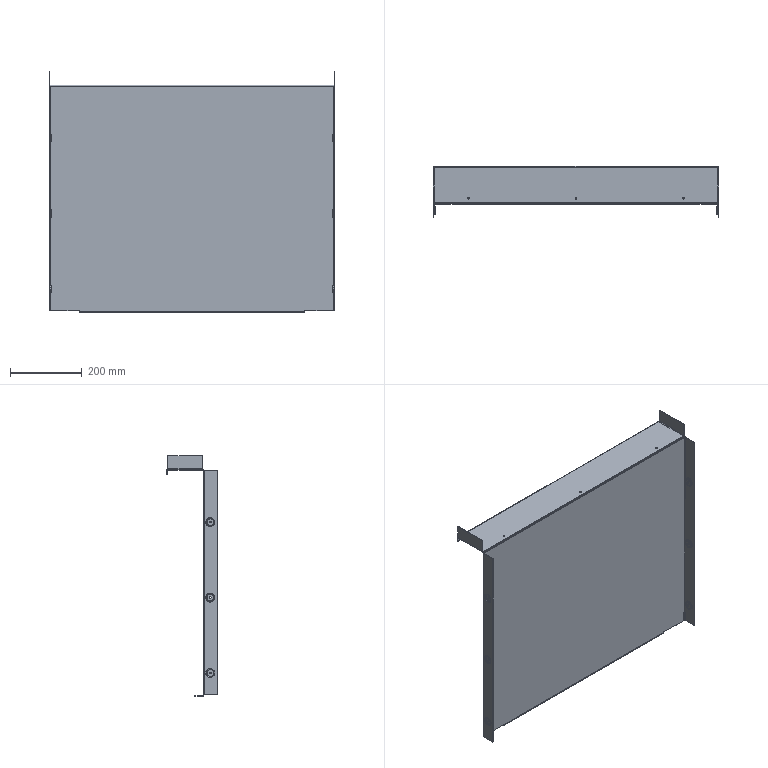Part | STEP file | 1 solid | 186 faces | box 795 x 142 x 670 mm | volume 1317860 mm3 | plane 70 | cylinder 68 | torus 48 | commonest cylinder face diameters 5.3 x18 4.7 x12 20 x12 24 x12 3 x7 7 x7